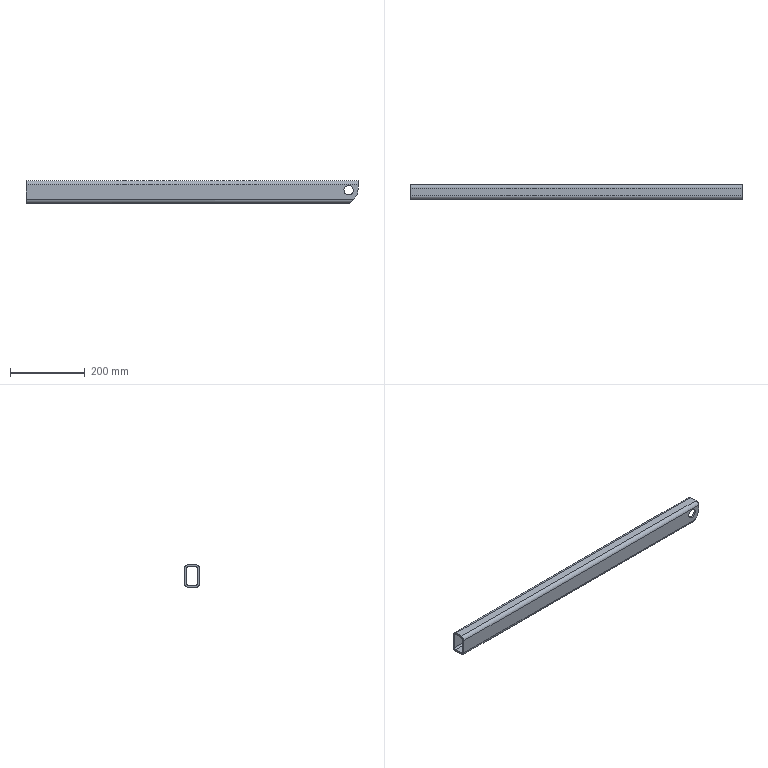Part | STEP file | frame crossmember 2-000.001--20240926 | 1 solid | 23 faces | box 887 x 40 x 60 mm | volume 731037 mm3 | cylinder 12 | plane 11 | commonest cylinder face diameters 10 x4 20 x4 25 x2 70 x2